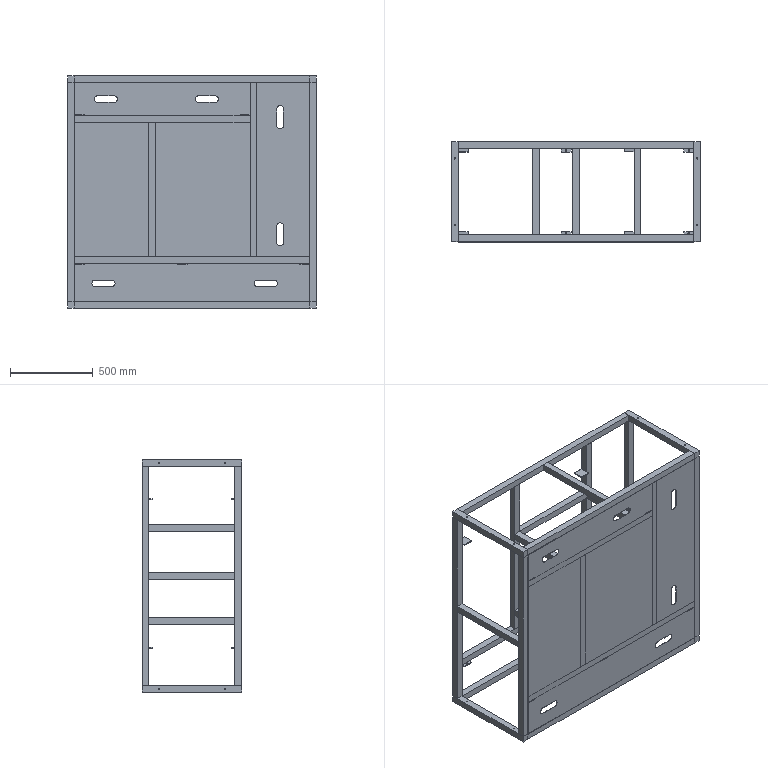Part | NX | features BREP 37 | 37 solids | 336 faces | box 1500 x 602 x 1400 mm | volume 46380965 mm3 | plane 246 | cylinder 90 | commonest cylinder face diameters 7 x64 40 x14 9.834 x2 10.72 x2 10.905 x2 11.377 x2